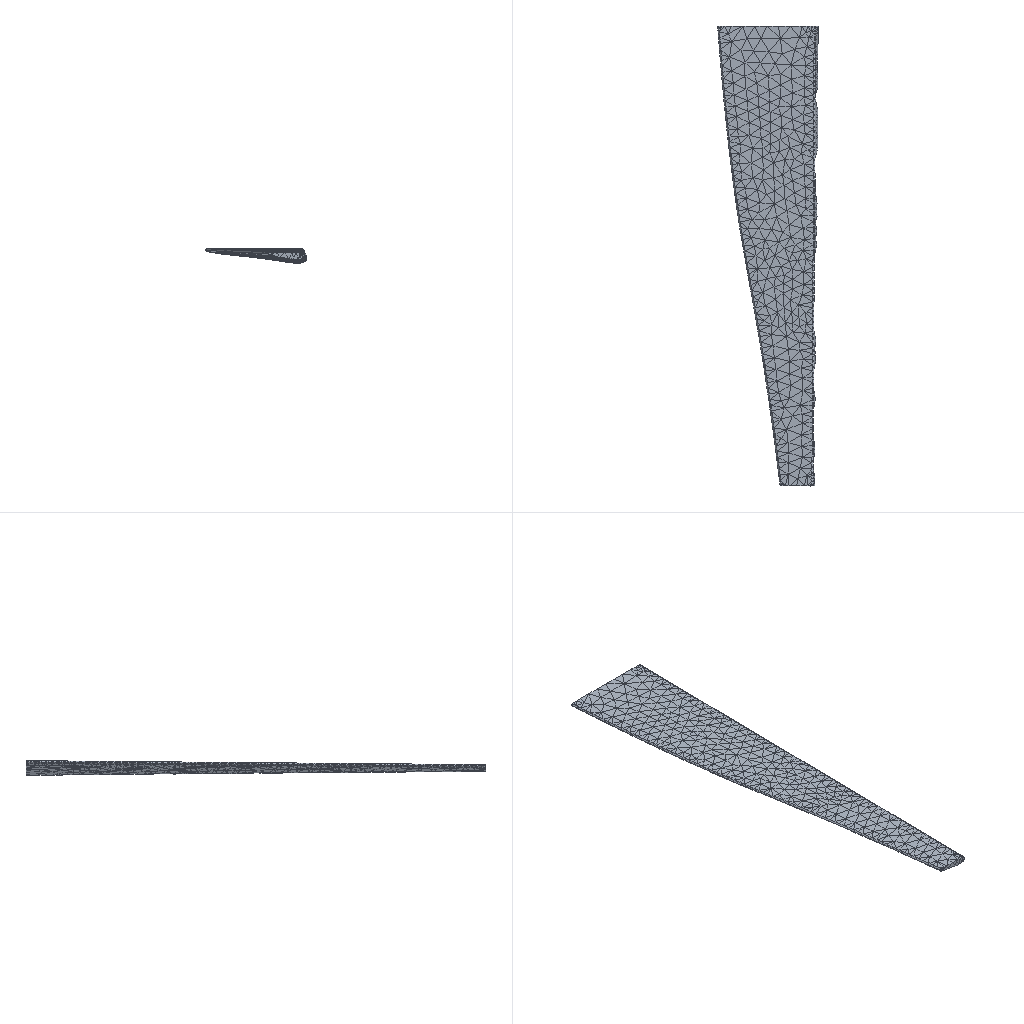Simulation study | ansys workbench
Set-up summary:
category,name,step,type,value,unit,region
solver,ansys_workbench
units,mm-N-s-tonne (MPa),,stated,"/units,MPA"
analysis,LS1,,static
load_step,LS1,LS1,static,nsubst=1; time=1
mesh,nodes,,,6118
mesh,elements,,,4697
element_type,SOLID187,,,2960
element_type,SURF154,,,1737
material,Structural Steel,,E,200000,tonne s^-2 mm^-1
material,Structural Steel,,nu,0.3
material,Structural Steel,,density,7.85e-09,tonne mm^-3
material,Structural Steel,,conductivity,60.5,tonne mm s^-3 C^-1
material,Structural Steel,,specific_heat,4.34e+08,mm^2 s^-2 C^-1
material,Structural Steel,,cte,1.2e-05,C^-1
material,Structural Steel,,permeability,10000
material,Structural Steel,,resistivity,0.00017,ohm mm
load,Define Force Using Surface Effect Elements,LS1,surface-effect pres face 1,411.025,,SURF154 #2
bc,Fixed Supports,model,fixed,[dofs=ALL],,_FIXEDSU
named_set,_FIXEDSU,,node,97
Ansys APDL input file, long lists of numbers shortened:
/batch
/config,noeldb,1     ! force off writing results to database
*get,_wallstrt,active,,time,wall
! ANSYS input file written by Workbench version 2022 R1
! File used for geometry attach:
/title,wbnew--____ (B5)
! ****** Begin Custom Load Command Snippet ******
/COM, ACT Extensions:
/COM,     LSDYNA, 2021.1
/COM,
! ****** End   Custom Load Command Snippet ******
*DIM,_wb_ProjectScratch_dir,string,248
_wb_ProjectScratch_dir(1) = ''
*DIM,_wb_SolverFiles_dir,string,248
_wb_SolverFiles_dir(1) = ''
*DIM,_wb_userfiles_dir,string,248
_wb_userfiles_dir(1) = ''
/com,--- Data in consistent NMM units. See Solving Units in the help system for more information.
/units,MPA
/nopr
/wb,file,start              !  signify a WB generated input file
/prep7
! Turn off shape checking because checks already performed inside WB mesher.
! See help system for more information.
SHPP,OFF,,NOWARN
/nolist
etcon,set             ! allow ANSYS to choose best KEYOP's for 180x elements, resets any applicable keyopt to MAPDL defaults
/com,*********** Nodes for the whole assembly ***********
nblock,3,,6729
(1i9,3e20.9e3)
        1     1.474347104E+01    -6.500000000E+01    -6.715029459E-01
! (6117 more lines like these left out)
-1
/wb,elem,start            !  set before creation of elements
/com,*********** Elements for Body 1 "___6-FreeParts|__3" ***********
et,1,187
eblock,19,solid,,2960
(19i9)
        1        1        1        1        0        0        0        0       10        0        1        4        6      531     1089     1111     1126     1115     1117
! (5919 more lines like these left out)
-1
/wb,elem,end               !  done creating elements
/com,*********** Send User Defined Coordinate System(s) ***********
csys,0
toffst,273.15,  ! Temperature offset from absolute zero
/com,*********** Set Reference Temperature ***********
tref,22.
/wb,mat,start              !  starting to send materials
/com,*********** Send Materials ***********
Temperature = 'TEMP' ! Temperature
MP,DENS,1,7.85e-09,	! tonne mm^-3
MP,ALPX,1,1.2e-05,	! C^-1
MP,C,1,434000000,	! mm^2 s^-2 C^-1
MP,KXX,1,60.5,	! tonne mm s^-3 C^-1
MP,RSVX,1,0.00017,	! ohm mm
MP,EX,1,200000,	! tonne s^-2 mm^-1
MP,NUXY,1,0.3,
MP,MURX,1,10000,
/wb,mat,end                !  done sending materials
!************************* Model Summary ********************
!___6-FreeParts|__3,	结构钢,	matid,	1
!************************* End Model Summary ********************
! get the diagonal of the bounding box. Needed later for other things
*get,_xmin,node,,mnloc,x
*get,_ymin,node,,mnloc,y
*get,_zmin,node,,mnloc,z
*get,_xmax,node,,mxloc,x
*get,_ymax,node,,mxloc,y
*get,_zmax,node,,mxloc,z
_ASMDIAG=(_xmax-_xmin)*(_xmax-_xmin)+(_ymax-_ymin)*(_ymax-_ymin)+(_zmax-_zmin)*(_zmax-_zmin)
_ASMDIAG=SQRT(_ASMDIAG)
/wb,contact,start          !  starting to send contact
/wb,contact,end            !  done creating contacts
/golist
/wb,load,start             !  starting to send loads
/com,*********** Fixed Supports ***********
CMBLOCK,_FIXEDSU,NODE,       97
(8i10)
         7        27        28        29        30        31        32        33
! (12 more lines like these left out)
cmsel,s,_FIXEDSU
d,all,all
nsel,all
/com,*********** Define Force Using Surface Effect Elements ***********
local,12,0,0.,0.,0.,0.,0.,0.
csys,0
et,2,154
eblock,10,,,1737
(15i9)
     4919        2        2        2       12      814      854      815      815     5632     5639      815     5631
! (1736 more lines like these left out)
-1
esel,s,type,,2
keyop,2,2,1                ! Apply load in local coordinate system
keyop,2,7,1                ! Use original area so load is constant in large deformation
esel,all
/gst,on,on
fini
*get,_numnode,node,0,count
*get,_numelem,elem,0,count
*get, _MAXELEMNUM, elem, 0, NUM, MAX
*get, _MAXNODENUM, node, 0, NUM, MAX
*get, _MAXELEMTYPE, etyp, 0, NUM, MAX
*get, _MAXREALCONST, real, 0, NUM, MAX
/go
/wb,load,end               !  done creating loads
/com,--- Number of total nodes = %_numnode%
/com,--- Number of contact elements = 1737
/com,--- Number of spring elements = 0
/com,--- Number of bearing elements = 0
/com,--- Number of solid elements = 2960
/com,--- Number of condensed parts = 0
/com,--- Number of total elements = %_numelem%
*get,_wallbsol,active,,time,wall
/com,****************************************************************************
/com,*************************    SOLUTION       ********************************
/com,****************************************************************************
/solu
antype,0                   ! static analysis
_thickRatio=  0     ! Ratio of thick parts in the model
eqsl,sparse,,,,,1
cntr,print,1               ! print out contact info and also make no initial contact an error
dmpoption,emat,no             ! Don't combine emat file for DANSYS
dmpoption,esav,no             ! Don't combine esav file for DANSYS
nldiag,cont,iter           ! print out contact info each equilibrium iteration
rescontrol,,none                 ! Do not keep any restart files
/com,****************************************************
/com,******************* SOLVE FOR LS 1 OF 1 ****************
esel,s,type,,2
nsle
sfe,all,1,pres,1,411.025
sfe,all,2,pres,1,0.
sfe,all,3,pres,1,0.
nsel,all
esel,all
/nopr
/gopr
nsub,1,1,1
time,1.
outres,erase
outres,all,none
outres,nsol,all,
outres,rsol,all
outres,eangl,all
outres,etmp,all
outres,veng,all
outres,strs,all,
outres,epel,all,
outres,eppl,all,
outres,cont,all,
! *********** WB SOLVE COMMAND ***********
! check interactive state
*get,ANSINTER_,active,,int
*if,ANSINTER_,ne,0,then
/eof
*endif
solve
/com *************** Write FE CONNECTORS *********
CEWRITE,file,ce,,INTE
/com,****************************************************
/com,*************** FINISHED SOLVE FOR LS 1 *************
*get,_wallasol,active,,time,wall
/nopr
*get,_numnode,node,0,count
*get,_numelem,elem,0,count
*get, _MAXELEMNUM, elem, 0, NUM, MAX
*get, _MAXNODENUM, node, 0, NUM, MAX,,,INTERNAL
*get, _MAXELEMTYPE, etyp, 0, NUM, MAX
*get, _MAXREALCONST, real, 0, NUM, MAX
/gopr
/post1
xmlo,ENCODING,ISO-8859-1
xmlo,parm
/xml,parm,xml
fini
/gopr
*get,_walldone,active,,time,wall
_preptime=(_wallbsol-_wallstrt)*3600
_solvtime=(_wallasol-_wallbsol)*3600
_posttime=(_walldone-_wallasol)*3600
_totaltim=(_walldone-_wallstrt)*3600
*get,_dlbratio,active,0,solu,dlbr
*get,_combtime,active,0,solu,comb
*get,_ssmode,active,0,solu,ssmm
*get,_ndofs,active,0,solu,ndof
*get,_sol_end_time,active,0,set,time
*if,_sol_end_time,eq,1.,then
/fclean				!clean distributed files
*endif
/com,--- Total number of nodes = %_numnode%
/com,--- Total number of elements = %_numelem%
/com,--- Element load balance ratio = %_dlbratio%
/com,--- Time to combine distributed files = %_combtime%
/com,--- Sparse memory mode = %_ssmode%
/com,--- Number of DOF = %_ndofs%
/wb,file,end               ! done with WB generated input
Results summary:
result,analyses[0].index,,,1
result,analyses[0].system,,,SYS
result,analyses[0].deck,,,deck.dat
result,analyses[0].solve_status,,,completed
result,analyses[0].analysis_type,,,static
result,analyses[0].physics,,,mechanical
result,analyses[0].unit_system,,,"NMM: mm, ton, N, s, mV, mA, degC"
result,analyses[0].n_sets,,,1
result,analyses[0].load_steps[0].set,set=1,,1
result,analyses[0].load_steps[0].time_or_freq,set=1,,1
result,analyses[0].load_steps[0].max_displacement_magnitude,set=1,,2153.5
result,analyses[0].load_steps[0].max_von_mises_nodal,set=1,,765604
result,analyses[0].load_steps[0].reaction_force_sum_xyz[1],set=1,,-554972
result,analyses[0].load_steps[0].reaction_force_sum_xyz[2],set=1,,4.87875e-07
result,analyses[0].load_steps[0].reaction_force_sum_xyz[3],set=1,,-6.11872e-07